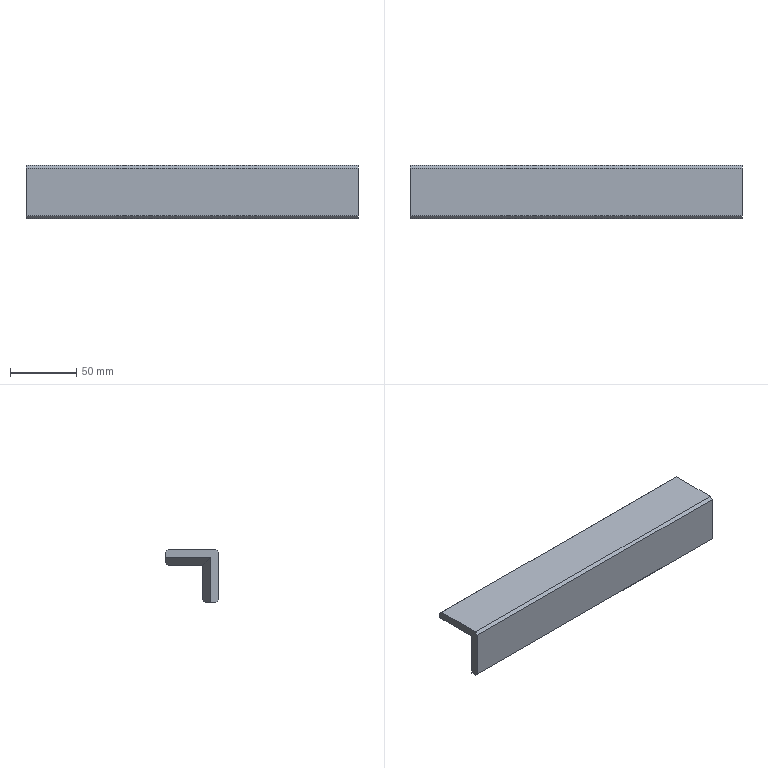Part | NX | 1 solid | 23 faces | box 250 x 40 x 40 mm | volume 198881 mm3 | plane 15 | cone 4 | cylinder 4 | commonest cylinder face diameters 4.2 x4
STEP:
#1=CARTESIAN_POINT('',(125.,-18.,20.));
#2=VERTEX_POINT('',#1);
#3=CARTESIAN_POINT('',(125.,-20.,18.));
#4=VERTEX_POINT('',#3);
#5=CARTESIAN_POINT('',(125.,-19.,19.));
#6=DIRECTION('',(0.,-0.7071,-0.7071));
#7=VECTOR('',#6,1000.);
#8=LINE('',#5,#7);
#9=EDGE_CURVE('',#2,#4,#8,.T.);
#10=ORIENTED_EDGE('',*,*,#9,.F.);
#11=CARTESIAN_POINT('',(-125.,-18.,20.));
#12=VERTEX_POINT('',#11);
#13=CARTESIAN_POINT('',(125.,-18.,20.));
#14=DIRECTION('',(1.,0.,0.));
#15=VECTOR('',#14,1000.);
#16=LINE('',#13,#15);
#17=EDGE_CURVE('',#12,#2,#16,.T.);
#18=ORIENTED_EDGE('',*,*,#17,.F.);
#19=CARTESIAN_POINT('',(-125.,-20.,18.));
#20=VERTEX_POINT('',#19);
#21=CARTESIAN_POINT('',(-125.,-20.,18.));
#22=DIRECTION('',(0.,0.7071,0.7071));
#23=VECTOR('',#22,1000.);
#24=LINE('',#21,#23);
#25=EDGE_CURVE('',#20,#12,#24,.T.);
#26=ORIENTED_EDGE('',*,*,#25,.F.);
#27=CARTESIAN_POINT('',(125.,-20.,18.));
#28=DIRECTION('',(-1.,0.,0.));
#29=VECTOR('',#28,1000.);
#30=LINE('',#27,#29);
#31=EDGE_CURVE('',#4,#20,#30,.T.);
#32=ORIENTED_EDGE('',*,*,#31,.F.);
#33=EDGE_LOOP('',(#10,#18,#26,#32));
#34=FACE_BOUND('',#33,.T.);
#35=CARTESIAN_POINT('',(125.,-20.,18.));
#36=DIRECTION('',(0.,0.7071,-0.7071));
#37=DIRECTION('',(-1.,0.,0.));
#38=AXIS2_PLACEMENT_3D('',#35,#36,#37);
#39=PLANE('',#38);
#40=ADVANCED_FACE('',(#34),#39,.F.);
#41=CARTESIAN_POINT('',(125.,-20.,-18.));
#42=VERTEX_POINT('',#41);
#43=CARTESIAN_POINT('',(125.,-18.,-20.));
#44=VERTEX_POINT('',#43);
#45=CARTESIAN_POINT('',(125.,-19.,-19.));
#46=DIRECTION('',(0.,0.7071,-0.7071));
#47=VECTOR('',#46,1000.);
#48=LINE('',#45,#47);
#49=EDGE_CURVE('',#42,#44,#48,.T.);
#50=ORIENTED_EDGE('',*,*,#49,.F.);
#51=CARTESIAN_POINT('',(-125.,-20.,-18.));
#52=VERTEX_POINT('',#51);
#53=CARTESIAN_POINT('',(125.,-20.,-18.));
#54=DIRECTION('',(1.,0.,0.));
#55=VECTOR('',#54,1000.);
#56=LINE('',#53,#55);
#57=EDGE_CURVE('',#52,#42,#56,.T.);
#58=ORIENTED_EDGE('',*,*,#57,.F.);
#59=CARTESIAN_POINT('',(-125.,-18.,-20.));
#60=VERTEX_POINT('',#59);
#61=CARTESIAN_POINT('',(-125.,-18.,-20.));
#62=DIRECTION('',(0.,-0.7071,0.7071));
#63=VECTOR('',#62,1000.);
#64=LINE('',#61,#63);
#65=EDGE_CURVE('',#60,#52,#64,.T.);
#66=ORIENTED_EDGE('',*,*,#65,.F.);
#67=CARTESIAN_POINT('',(125.,-18.,-20.));
#68=DIRECTION('',(-1.,0.,0.));
#69=VECTOR('',#68,1000.);
#70=LINE('',#67,#69);
#71=EDGE_CURVE('',#44,#60,#70,.T.);
#72=ORIENTED_EDGE('',*,*,#71,.F.);
#73=EDGE_LOOP('',(#50,#58,#66,#72));
#74=FACE_BOUND('',#73,.T.);
#75=CARTESIAN_POINT('',(125.,-18.,-20.));
#76=DIRECTION('',(0.,0.7071,0.7071));
#77=DIRECTION('',(-1.,0.,0.));
#78=AXIS2_PLACEMENT_3D('',#75,#76,#77);
#79=PLANE('',#78);
#80=ADVANCED_FACE('',(#74),#79,.F.);
#81=CARTESIAN_POINT('',(125.,20.,18.));
#82=VERTEX_POINT('',#81);
#83=CARTESIAN_POINT('',(125.,18.,20.));
#84=VERTEX_POINT('',#83);
#85=CARTESIAN_POINT('',(125.,19.,19.));
#86=DIRECTION('',(0.,-0.7071,0.7071));
#87=VECTOR('',#86,1000.);
#88=LINE('',#85,#87);
#89=EDGE_CURVE('',#82,#84,#88,.T.);
#90=ORIENTED_EDGE('',*,*,#89,.F.);
#91=CARTESIAN_POINT('',(-125.,20.,18.));
#92=VERTEX_POINT('',#91);
#93=CARTESIAN_POINT('',(125.,20.,18.));
#94=DIRECTION('',(1.,0.,0.));
#95=VECTOR('',#94,1000.);
#96=LINE('',#93,#95);
#97=EDGE_CURVE('',#92,#82,#96,.T.);
#98=ORIENTED_EDGE('',*,*,#97,.F.);
#99=CARTESIAN_POINT('',(-125.,18.,20.));
#100=VERTEX_POINT('',#99);
#101=CARTESIAN_POINT('',(-125.,18.,20.));
#102=DIRECTION('',(0.,0.7071,-0.7071));
#103=VECTOR('',#102,1000.);
#104=LINE('',#101,#103);
#105=EDGE_CURVE('',#100,#92,#104,.T.);
#106=ORIENTED_EDGE('',*,*,#105,.F.);
#107=CARTESIAN_POINT('',(125.,18.,20.));
#108=DIRECTION('',(-1.,0.,0.));
#109=VECTOR('',#108,1000.);
#110=LINE('',#107,#109);
#111=EDGE_CURVE('',#84,#100,#110,.T.);
#112=ORIENTED_EDGE('',*,*,#111,.F.);
#113=EDGE_LOOP('',(#90,#98,#106,#112));
#114=FACE_BOUND('',#113,.T.);
#115=CARTESIAN_POINT('',(125.,18.,20.));
#116=DIRECTION('',(0.,-0.7071,-0.7071));
#117=DIRECTION('',(-1.,0.,0.));
#118=AXIS2_PLACEMENT_3D('',#115,#116,#117);
#119=PLANE('',#118);
#120=ADVANCED_FACE('',(#114),#119,.F.);
#121=CARTESIAN_POINT('',(-118.333,20.,10.));
#122=VERTEX_POINT('',#121);
#123=CARTESIAN_POINT('',(-115.,18.,8.));
#124=VERTEX_POINT('',#123);
#125=CARTESIAN_POINT('',(-116.628,18.977,8.977));
#126=DIRECTION('',(0.7625,-0.4575,-0.4575));
#127=VECTOR('',#126,1000.);
#128=LINE('',#125,#127);
#129=EDGE_CURVE('',#122,#124,#128,.T.);
#130=ORIENTED_EDGE('',*,*,#129,.F.);
#131=CARTESIAN_POINT('',(125.,20.,10.));
#132=VERTEX_POINT('',#131);
#133=CARTESIAN_POINT('',(125.,20.,10.));
#134=DIRECTION('',(-1.,0.,0.));
#135=VECTOR('',#134,1000.);
#136=LINE('',#133,#135);
#137=EDGE_CURVE('',#132,#122,#136,.T.);
#138=ORIENTED_EDGE('',*,*,#137,.F.);
#139=CARTESIAN_POINT('',(125.,18.,8.));
#140=VERTEX_POINT('',#139);
#141=CARTESIAN_POINT('',(125.,5.,-5.));
#142=DIRECTION('',(0.,0.7071,0.7071));
#143=VECTOR('',#142,1000.);
#144=LINE('',#141,#143);
#145=EDGE_CURVE('',#140,#132,#144,.T.);
#146=ORIENTED_EDGE('',*,*,#145,.F.);
#147=CARTESIAN_POINT('',(-125.,18.,8.));
#148=DIRECTION('',(1.,0.,0.));
#149=VECTOR('',#148,1000.);
#150=LINE('',#147,#149);
#151=EDGE_CURVE('',#124,#140,#150,.T.);
#152=ORIENTED_EDGE('',*,*,#151,.F.);
#153=EDGE_LOOP('',(#130,#138,#146,#152));
#154=FACE_BOUND('',#153,.T.);
#155=CARTESIAN_POINT('',(125.,-10.,-20.));
#156=DIRECTION('',(0.,-0.7071,0.7071));
#157=DIRECTION('',(1.,0.,0.));
#158=AXIS2_PLACEMENT_3D('',#155,#156,#157);
#159=PLANE('',#158);
#160=ADVANCED_FACE('',(#154),#159,.F.);
#161=CARTESIAN_POINT('',(-115.,-8.,-18.));
#162=VERTEX_POINT('',#161);
#163=CARTESIAN_POINT('',(-118.333,-10.,-20.));
#164=VERTEX_POINT('',#163);
#165=CARTESIAN_POINT('',(-116.628,-8.977,-18.977));
#166=DIRECTION('',(-0.7625,-0.4575,-0.4575));
#167=VECTOR('',#166,1000.);
#168=LINE('',#165,#167);
#169=EDGE_CURVE('',#162,#164,#168,.T.);
#170=ORIENTED_EDGE('',*,*,#169,.F.);
#171=CARTESIAN_POINT('',(125.,-8.,-18.));
#172=VERTEX_POINT('',#171);
#173=CARTESIAN_POINT('',(-125.,-8.,-18.));
#174=DIRECTION('',(-1.,0.,0.));
#175=VECTOR('',#174,1000.);
#176=LINE('',#173,#175);
#177=EDGE_CURVE('',#172,#162,#176,.T.);
#178=ORIENTED_EDGE('',*,*,#177,.F.);
#179=CARTESIAN_POINT('',(125.,-10.,-20.));
#180=VERTEX_POINT('',#179);
#181=CARTESIAN_POINT('',(125.,5.,-5.));
#182=DIRECTION('',(0.,0.7071,0.7071));
#183=VECTOR('',#182,1000.);
#184=LINE('',#181,#183);
#185=EDGE_CURVE('',#180,#172,#184,.T.);
#186=ORIENTED_EDGE('',*,*,#185,.F.);
#187=CARTESIAN_POINT('',(125.,-10.,-20.));
#188=DIRECTION('',(1.,0.,0.));
#189=VECTOR('',#188,1000.);
#190=LINE('',#187,#189);
#191=EDGE_CURVE('',#164,#180,#190,.T.);
#192=ORIENTED_EDGE('',*,*,#191,.F.);
#193=EDGE_LOOP('',(#170,#178,#186,#192));
#194=FACE_BOUND('',#193,.T.);
#195=CARTESIAN_POINT('',(125.,-10.,-20.));
#196=DIRECTION('',(0.,-0.7071,0.7071));
#197=DIRECTION('',(1.,0.,0.));
#198=AXIS2_PLACEMENT_3D('',#195,#196,#197);
#199=PLANE('',#198);
#200=ADVANCED_FACE('',(#194),#199,.F.);
#201=CARTESIAN_POINT('',(-115.,-8.,8.));
#202=VERTEX_POINT('',#201);
#203=CARTESIAN_POINT('',(-115.,-8.,-20.));
#204=DIRECTION('',(0.,0.,1.));
#205=VECTOR('',#204,1000.);
#206=LINE('',#203,#205);
#207=EDGE_CURVE('',#162,#202,#206,.T.);
#208=ORIENTED_EDGE('',*,*,#207,.F.);
#209=ORIENTED_EDGE('',*,*,#169,.T.);
#210=CARTESIAN_POINT('',(-125.,-14.,-20.));
#211=VERTEX_POINT('',#210);
#212=CARTESIAN_POINT('',(-125.,-14.,-20.));
#213=DIRECTION('',(0.8575,0.5145,0.));
#214=VECTOR('',#213,1000.);
#215=LINE('',#212,#214);
#216=EDGE_CURVE('',#211,#164,#215,.T.);
#217=ORIENTED_EDGE('',*,*,#216,.F.);
#218=CARTESIAN_POINT('',(-125.,-14.,14.));
#219=VERTEX_POINT('',#218);
#220=CARTESIAN_POINT('',(-125.,-14.,0.));
#221=DIRECTION('',(0.,0.,-1.));
#222=VECTOR('',#221,1000.);
#223=LINE('',#220,#222);
#224=EDGE_CURVE('',#219,#211,#223,.T.);
#225=ORIENTED_EDGE('',*,*,#224,.F.);
#226=CARTESIAN_POINT('',(-120.116,-11.07,11.07));
#227=DIRECTION('',(0.7625,0.4575,-0.4575));
#228=VECTOR('',#227,1000.);
#229=LINE('',#226,#228);
#230=EDGE_CURVE('',#219,#202,#229,.T.);
#231=ORIENTED_EDGE('',*,*,#230,.T.);
#232=EDGE_LOOP('',(#208,#209,#217,#225,#231));
#233=FACE_BOUND('',#232,.T.);
#234=CARTESIAN_POINT('',(-125.,-14.,0.));
#235=DIRECTION('',(0.5145,-0.8575,0.));
#236=DIRECTION('',(0.,0.,-1.));
#237=AXIS2_PLACEMENT_3D('',#234,#235,#236);
#238=PLANE('',#237);
#239=ADVANCED_FACE('',(#233),#238,.F.);
#240=CARTESIAN_POINT('',(-125.,20.,14.));
#241=VERTEX_POINT('',#240);
#242=CARTESIAN_POINT('',(-125.,20.,14.));
#243=DIRECTION('',(-0.8575,0.,0.5145));
#244=VECTOR('',#243,1000.);
#245=LINE('',#242,#244);
#246=EDGE_CURVE('',#122,#241,#245,.T.);
#247=ORIENTED_EDGE('',*,*,#246,.F.);
#248=ORIENTED_EDGE('',*,*,#129,.T.);
#249=CARTESIAN_POINT('',(-115.,20.,8.));
#250=DIRECTION('',(0.,1.,0.));
#251=VECTOR('',#250,1000.);
#252=LINE('',#249,#251);
#253=EDGE_CURVE('',#202,#124,#252,.T.);
#254=ORIENTED_EDGE('',*,*,#253,.F.);
#255=ORIENTED_EDGE('',*,*,#230,.F.);
#256=CARTESIAN_POINT('',(-125.,0.,14.));
#257=DIRECTION('',(0.,-1.,0.));
#258=VECTOR('',#257,1000.);
#259=LINE('',#256,#258);
#260=EDGE_CURVE('',#241,#219,#259,.T.);
#261=ORIENTED_EDGE('',*,*,#260,.F.);
#262=EDGE_LOOP('',(#247,#248,#254,#255,#261));
#263=FACE_BOUND('',#262,.T.);
#264=CARTESIAN_POINT('',(-125.,0.,14.));
#265=DIRECTION('',(0.5145,0.,0.8575));
#266=DIRECTION('',(0.,-1.,0.));
#267=AXIS2_PLACEMENT_3D('',#264,#265,#266);
#268=PLANE('',#267);
#269=ADVANCED_FACE('',(#263),#268,.F.);
#270=ORIENTED_EDGE('',*,*,#253,.T.);
#271=ORIENTED_EDGE('',*,*,#151,.T.);
#272=CARTESIAN_POINT('',(125.,-8.,8.));
#273=VERTEX_POINT('',#272);
#274=CARTESIAN_POINT('',(125.,20.,8.));
#275=DIRECTION('',(0.,-1.,0.));
#276=VECTOR('',#275,1000.);
#277=LINE('',#274,#276);
#278=EDGE_CURVE('',#140,#273,#277,.T.);
#279=ORIENTED_EDGE('',*,*,#278,.T.);
#280=CARTESIAN_POINT('',(-125.,-8.,8.));
#281=DIRECTION('',(1.,0.,0.));
#282=VECTOR('',#281,1000.);
#283=LINE('',#280,#282);
#284=EDGE_CURVE('',#202,#273,#283,.T.);
#285=ORIENTED_EDGE('',*,*,#284,.F.);
#286=EDGE_LOOP('',(#270,#271,#279,#285));
#287=FACE_BOUND('',#286,.T.);
#288=CARTESIAN_POINT('',(-125.,20.,8.));
#289=DIRECTION('',(0.,0.,1.));
#290=DIRECTION('',(0.,-1.,0.));
#291=AXIS2_PLACEMENT_3D('',#288,#289,#290);
#292=PLANE('',#291);
#293=ADVANCED_FACE('',(#287),#292,.F.);
#294=CARTESIAN_POINT('',(125.,-8.,-20.));
#295=DIRECTION('',(0.,0.,-1.));
#296=VECTOR('',#295,1000.);
#297=LINE('',#294,#296);
#298=EDGE_CURVE('',#273,#172,#297,.T.);
#299=ORIENTED_EDGE('',*,*,#298,.T.);
#300=ORIENTED_EDGE('',*,*,#177,.T.);
#301=ORIENTED_EDGE('',*,*,#207,.T.);
#302=ORIENTED_EDGE('',*,*,#284,.T.);
#303=EDGE_LOOP('',(#299,#300,#301,#302));
#304=FACE_BOUND('',#303,.T.);
#305=CARTESIAN_POINT('',(-125.,-8.,-20.));
#306=DIRECTION('',(0.,-1.,0.));
#307=DIRECTION('',(0.,0.,-1.));
#308=AXIS2_PLACEMENT_3D('',#305,#306,#307);
#309=PLANE('',#308);
#310=ADVANCED_FACE('',(#304),#309,.F.);
#311=CARTESIAN_POINT('',(-125.,20.,20.));
#312=DIRECTION('',(0.,-1.,0.));
#313=VECTOR('',#312,1000.);
#314=LINE('',#311,#313);
#315=EDGE_CURVE('',#100,#12,#314,.T.);
#316=ORIENTED_EDGE('',*,*,#315,.F.);
#317=ORIENTED_EDGE('',*,*,#105,.T.);
#318=CARTESIAN_POINT('',(-125.,20.,20.));
#319=DIRECTION('',(0.,0.,1.));
#320=VECTOR('',#319,1000.);
#321=LINE('',#318,#320);
#322=EDGE_CURVE('',#241,#92,#321,.T.);
#323=ORIENTED_EDGE('',*,*,#322,.F.);
#324=ORIENTED_EDGE('',*,*,#260,.T.);
#325=ORIENTED_EDGE('',*,*,#224,.T.);
#326=CARTESIAN_POINT('',(-125.,20.,-20.));
#327=DIRECTION('',(0.,1.,0.));
#328=VECTOR('',#327,1000.);
#329=LINE('',#326,#328);
#330=EDGE_CURVE('',#60,#211,#329,.T.);
#331=ORIENTED_EDGE('',*,*,#330,.F.);
#332=ORIENTED_EDGE('',*,*,#65,.T.);
#333=CARTESIAN_POINT('',(-125.,-20.,20.));
#334=DIRECTION('',(0.,0.,-1.));
#335=VECTOR('',#334,1000.);
#336=LINE('',#333,#335);
#337=EDGE_CURVE('',#20,#52,#336,.T.);
#338=ORIENTED_EDGE('',*,*,#337,.F.);
#339=ORIENTED_EDGE('',*,*,#25,.T.);
#340=EDGE_LOOP('',(#316,#317,#323,#324,#325,#331,#332,#338,#339));
#341=FACE_BOUND('',#340,.T.);
#342=CARTESIAN_POINT('',(-125.,0.,0.));
#343=DIRECTION('',(1.,0.,0.));
#344=DIRECTION('',(0.,0.,-1.));
#345=AXIS2_PLACEMENT_3D('',#342,#343,#344);
#346=PLANE('',#345);
#347=ADVANCED_FACE('',(#341),#346,.F.);
#348=CARTESIAN_POINT('',(125.,20.,-20.));
#349=DIRECTION('',(0.,1.,0.));
#350=VECTOR('',#349,1000.);
#351=LINE('',#348,#350);
#352=EDGE_CURVE('',#44,#180,#351,.T.);
#353=ORIENTED_EDGE('',*,*,#352,.T.);
#354=ORIENTED_EDGE('',*,*,#185,.T.);
#355=ORIENTED_EDGE('',*,*,#298,.F.);
#356=ORIENTED_EDGE('',*,*,#278,.F.);
#357=ORIENTED_EDGE('',*,*,#145,.T.);
#358=CARTESIAN_POINT('',(125.,20.,20.));
#359=DIRECTION('',(0.,0.,1.));
#360=VECTOR('',#359,1000.);
#361=LINE('',#358,#360);
#362=EDGE_CURVE('',#132,#82,#361,.T.);
#363=ORIENTED_EDGE('',*,*,#362,.T.);
#364=ORIENTED_EDGE('',*,*,#89,.T.);
#365=CARTESIAN_POINT('',(125.,20.,20.));
#366=DIRECTION('',(0.,-1.,0.));
#367=VECTOR('',#366,1000.);
#368=LINE('',#365,#367);
#369=EDGE_CURVE('',#84,#2,#368,.T.);
#370=ORIENTED_EDGE('',*,*,#369,.T.);
#371=ORIENTED_EDGE('',*,*,#9,.T.);
#372=CARTESIAN_POINT('',(125.,-20.,20.));
#373=DIRECTION('',(0.,0.,-1.));
#374=VECTOR('',#373,1000.);
#375=LINE('',#372,#374);
#376=EDGE_CURVE('',#4,#42,#375,.T.);
#377=ORIENTED_EDGE('',*,*,#376,.T.);
#378=ORIENTED_EDGE('',*,*,#49,.T.);
#379=EDGE_LOOP('',(#353,#354,#355,#356,#357,#363,#364,#370,#371,#377,#378));
#380=FACE_BOUND('',#379,.T.);
#381=CARTESIAN_POINT('',(125.,14.,11.9));
#382=VERTEX_POINT('',#381);
#383=CARTESIAN_POINT('',(125.,14.,14.));
#384=DIRECTION('',(1.,0.,0.));
#385=DIRECTION('',(0.,0.,-1.));
#386=AXIS2_PLACEMENT_3D('',#383,#384,#385);
#387=CIRCLE('',#386,2.1);
#388=EDGE_CURVE('',#382,#382,#387,.T.);
#389=ORIENTED_EDGE('',*,*,#388,.F.);
#390=EDGE_LOOP('',(#389));
#391=FACE_BOUND('',#390,.T.);
#392=CARTESIAN_POINT('',(125.,-2.,11.9));
#393=VERTEX_POINT('',#392);
#394=CARTESIAN_POINT('',(125.,-2.,14.));
#395=DIRECTION('',(1.,0.,0.));
#396=DIRECTION('',(0.,0.,-1.));
#397=AXIS2_PLACEMENT_3D('',#394,#395,#396);
#398=CIRCLE('',#397,2.1);
#399=EDGE_CURVE('',#393,#393,#398,.T.);
#400=ORIENTED_EDGE('',*,*,#399,.F.);
#401=EDGE_LOOP('',(#400));
#402=FACE_BOUND('',#401,.T.);
#403=CARTESIAN_POINT('',(125.,-14.,-0.1));
#404=VERTEX_POINT('',#403);
#405=CARTESIAN_POINT('',(125.,-14.,2.));
#406=DIRECTION('',(1.,0.,0.));
#407=DIRECTION('',(0.,0.,-1.));
#408=AXIS2_PLACEMENT_3D('',#405,#406,#407);
#409=CIRCLE('',#408,2.1);
#410=EDGE_CURVE('',#404,#404,#409,.T.);
#411=ORIENTED_EDGE('',*,*,#410,.F.);
#412=EDGE_LOOP('',(#411));
#413=FACE_BOUND('',#412,.T.);
#414=CARTESIAN_POINT('',(125.,-14.,-16.1));
#415=VERTEX_POINT('',#414);
#416=CARTESIAN_POINT('',(125.,-14.,-14.));
#417=DIRECTION('',(1.,0.,0.));
#418=DIRECTION('',(0.,0.,-1.));
#419=AXIS2_PLACEMENT_3D('',#416,#417,#418);
#420=CIRCLE('',#419,2.1);
#421=EDGE_CURVE('',#415,#415,#420,.T.);
#422=ORIENTED_EDGE('',*,*,#421,.F.);
#423=EDGE_LOOP('',(#422));
#424=FACE_BOUND('',#423,.T.);
#425=CARTESIAN_POINT('',(125.,0.,0.));
#426=DIRECTION('',(1.,0.,0.));
#427=DIRECTION('',(0.,0.,-1.));
#428=AXIS2_PLACEMENT_3D('',#425,#426,#427);
#429=PLANE('',#428);
#430=ADVANCED_FACE('',(#380,#391,#402,#413,#424),#429,.T.);
#431=ORIENTED_EDGE('',*,*,#337,.T.);
#432=ORIENTED_EDGE('',*,*,#57,.T.);
#433=ORIENTED_EDGE('',*,*,#376,.F.);
#434=ORIENTED_EDGE('',*,*,#31,.T.);
#435=EDGE_LOOP('',(#431,#432,#433,#434));
#436=FACE_BOUND('',#435,.T.);
#437=CARTESIAN_POINT('',(125.,-20.,20.));
#438=DIRECTION('',(0.,1.,0.));
#439=DIRECTION('',(0.,0.,1.));
#440=AXIS2_PLACEMENT_3D('',#437,#438,#439);
#441=PLANE('',#440);
#442=ADVANCED_FACE('',(#436),#441,.F.);
#443=ORIENTED_EDGE('',*,*,#369,.F.);
#444=ORIENTED_EDGE('',*,*,#111,.T.);
#445=ORIENTED_EDGE('',*,*,#315,.T.);
#446=ORIENTED_EDGE('',*,*,#17,.T.);
#447=EDGE_LOOP('',(#443,#444,#445,#446));
#448=FACE_BOUND('',#447,.T.);
#449=CARTESIAN_POINT('',(125.,20.,20.));
#450=DIRECTION('',(0.,0.,-1.));
#451=DIRECTION('',(0.,1.,0.));
#452=AXIS2_PLACEMENT_3D('',#449,#450,#451);
#453=PLANE('',#452);
#454=ADVANCED_FACE('',(#448),#453,.F.);
#455=ORIENTED_EDGE('',*,*,#362,.F.);
#456=ORIENTED_EDGE('',*,*,#137,.T.);
#457=ORIENTED_EDGE('',*,*,#246,.T.);
#458=ORIENTED_EDGE('',*,*,#322,.T.);
#459=ORIENTED_EDGE('',*,*,#97,.T.);
#460=EDGE_LOOP('',(#455,#456,#457,#458,#459));
#461=FACE_BOUND('',#460,.T.);
#462=CARTESIAN_POINT('',(125.,20.,20.));
#463=DIRECTION('',(0.,-1.,0.));
#464=DIRECTION('',(0.,0.,-1.));
#465=AXIS2_PLACEMENT_3D('',#462,#463,#464);
#466=PLANE('',#465);
#467=ADVANCED_FACE('',(#461),#466,.F.);
#468=ORIENTED_EDGE('',*,*,#216,.T.);
#469=ORIENTED_EDGE('',*,*,#191,.T.);
#470=ORIENTED_EDGE('',*,*,#352,.F.);
#471=ORIENTED_EDGE('',*,*,#71,.T.);
#472=ORIENTED_EDGE('',*,*,#330,.T.);
#473=EDGE_LOOP('',(#468,#469,#470,#471,#472));
#474=FACE_BOUND('',#473,.T.);
#475=CARTESIAN_POINT('',(125.,20.,-20.));
#476=DIRECTION('',(0.,0.,1.));
#477=DIRECTION('',(0.,-1.,0.));
#478=AXIS2_PLACEMENT_3D('',#475,#476,#477);
#479=PLANE('',#478);
#480=ADVANCED_FACE('',(#474),#479,.F.);
#481=CARTESIAN_POINT('',(108.738,14.,14.));
#482=VERTEX_POINT('',#481);
#483=VERTEX_LOOP('',#482);
#484=FACE_BOUND('',#483,.T.);
#485=CARTESIAN_POINT('',(110.,14.,11.9));
#486=VERTEX_POINT('',#485);
#487=CARTESIAN_POINT('',(110.,14.,14.));
#488=DIRECTION('',(1.,0.,0.));
#489=DIRECTION('',(0.,0.,-1.));
#490=AXIS2_PLACEMENT_3D('',#487,#488,#489);
#491=CIRCLE('',#490,2.1);
#492=EDGE_CURVE('',#486,#486,#491,.T.);
#493=ORIENTED_EDGE('',*,*,#492,.T.);
#494=EDGE_LOOP('',(#493));
#495=FACE_BOUND('',#494,.T.);
#496=CARTESIAN_POINT('',(110.,14.,14.));
#497=DIRECTION('',(1.,0.,0.));
#498=DIRECTION('',(0.,0.,-1.));
#499=AXIS2_PLACEMENT_3D('',#496,#497,#498);
#500=CONICAL_SURFACE('',#499,2.1,1.03);
#501=ADVANCED_FACE('',(#484,#495),#500,.F.);
#502=ORIENTED_EDGE('',*,*,#388,.T.);
#503=EDGE_LOOP('',(#502));
#504=FACE_BOUND('',#503,.T.);
#505=ORIENTED_EDGE('',*,*,#492,.F.);
#506=EDGE_LOOP('',(#505));
#507=FACE_BOUND('',#506,.T.);
#508=CARTESIAN_POINT('',(125.,14.,14.));
#509=DIRECTION('',(1.,0.,0.));
#510=DIRECTION('',(0.,0.,-1.));
#511=AXIS2_PLACEMENT_3D('',#508,#509,#510);
#512=CYLINDRICAL_SURFACE('',#511,2.1);
#513=ADVANCED_FACE('',(#504,#507),#512,.F.);
#514=CARTESIAN_POINT('',(108.738,-2.,14.));
#515=VERTEX_POINT('',#514);
#516=VERTEX_LOOP('',#515);
#517=FACE_BOUND('',#516,.T.);
#518=CARTESIAN_POINT('',(110.,-2.,11.9));
#519=VERTEX_POINT('',#518);
#520=CARTESIAN_POINT('',(110.,-2.,14.));
#521=DIRECTION('',(1.,0.,0.));
#522=DIRECTION('',(0.,0.,-1.));
#523=AXIS2_PLACEMENT_3D('',#520,#521,#522);
#524=CIRCLE('',#523,2.1);
#525=EDGE_CURVE('',#519,#519,#524,.T.);
#526=ORIENTED_EDGE('',*,*,#525,.T.);
#527=EDGE_LOOP('',(#526));
#528=FACE_BOUND('',#527,.T.);
#529=CARTESIAN_POINT('',(110.,-2.,14.));
#530=DIRECTION('',(1.,0.,0.));
#531=DIRECTION('',(0.,0.,-1.));
#532=AXIS2_PLACEMENT_3D('',#529,#530,#531);
#533=CONICAL_SURFACE('',#532,2.1,1.03);
#534=ADVANCED_FACE('',(#517,#528),#533,.F.);
#535=ORIENTED_EDGE('',*,*,#399,.T.);
#536=EDGE_LOOP('',(#535));
#537=FACE_BOUND('',#536,.T.);
#538=ORIENTED_EDGE('',*,*,#525,.F.);
#539=EDGE_LOOP('',(#538));
#540=FACE_BOUND('',#539,.T.);
#541=CARTESIAN_POINT('',(125.,-2.,14.));
#542=DIRECTION('',(1.,0.,0.));
#543=DIRECTION('',(0.,0.,-1.));
#544=AXIS2_PLACEMENT_3D('',#541,#542,#543);
#545=CYLINDRICAL_SURFACE('',#544,2.1);
#546=ADVANCED_FACE('',(#537,#540),#545,.F.);
#547=CARTESIAN_POINT('',(108.738,-14.,2.));
#548=VERTEX_POINT('',#547);
#549=VERTEX_LOOP('',#548);
#550=FACE_BOUND('',#549,.T.);
#551=CARTESIAN_POINT('',(110.,-14.,-0.1));
#552=VERTEX_POINT('',#551);
#553=CARTESIAN_POINT('',(110.,-14.,2.));
#554=DIRECTION('',(1.,0.,0.));
#555=DIRECTION('',(0.,0.,-1.));
#556=AXIS2_PLACEMENT_3D('',#553,#554,#555);
#557=CIRCLE('',#556,2.1);
#558=EDGE_CURVE('',#552,#552,#557,.T.);
#559=ORIENTED_EDGE('',*,*,#558,.T.);
#560=EDGE_LOOP('',(#559));
#561=FACE_BOUND('',#560,.T.);
#562=CARTESIAN_POINT('',(110.,-14.,2.));
#563=DIRECTION('',(1.,0.,0.));
#564=DIRECTION('',(0.,0.,-1.));
#565=AXIS2_PLACEMENT_3D('',#562,#563,#564);
#566=CONICAL_SURFACE('',#565,2.1,1.03);
#567=ADVANCED_FACE('',(#550,#561),#566,.F.);
#568=ORIENTED_EDGE('',*,*,#410,.T.);
#569=EDGE_LOOP('',(#568));
#570=FACE_BOUND('',#569,.T.);
#571=ORIENTED_EDGE('',*,*,#558,.F.);
#572=EDGE_LOOP('',(#571));
#573=FACE_BOUND('',#572,.T.);
#574=CARTESIAN_POINT('',(125.,-14.,2.));
#575=DIRECTION('',(1.,0.,0.));
#576=DIRECTION('',(0.,0.,-1.));
#577=AXIS2_PLACEMENT_3D('',#574,#575,#576);
#578=CYLINDRICAL_SURFACE('',#577,2.1);
#579=ADVANCED_FACE('',(#570,#573),#578,.F.);
#580=CARTESIAN_POINT('',(108.738,-14.,-14.));
#581=VERTEX_POINT('',#580);
#582=VERTEX_LOOP('',#581);
#583=FACE_BOUND('',#582,.T.);
#584=CARTESIAN_POINT('',(110.,-14.,-16.1));
#585=VERTEX_POINT('',#584);
#586=CARTESIAN_POINT('',(110.,-14.,-14.));
#587=DIRECTION('',(1.,0.,0.));
#588=DIRECTION('',(0.,0.,-1.));
#589=AXIS2_PLACEMENT_3D('',#586,#587,#588);
#590=CIRCLE('',#589,2.1);
#591=EDGE_CURVE('',#585,#585,#590,.T.);
#592=ORIENTED_EDGE('',*,*,#591,.T.);
#593=EDGE_LOOP('',(#592));
#594=FACE_BOUND('',#593,.T.);
#595=CARTESIAN_POINT('',(110.,-14.,-14.));
#596=DIRECTION('',(1.,0.,0.));
#597=DIRECTION('',(0.,0.,-1.));
#598=AXIS2_PLACEMENT_3D('',#595,#596,#597);
#599=CONICAL_SURFACE('',#598,2.1,1.03);
#600=ADVANCED_FACE('',(#583,#594),#599,.F.);
#601=ORIENTED_EDGE('',*,*,#421,.T.);
#602=EDGE_LOOP('',(#601));
#603=FACE_BOUND('',#602,.T.);
#604=ORIENTED_EDGE('',*,*,#591,.F.);
#605=EDGE_LOOP('',(#604));
#606=FACE_BOUND('',#605,.T.);
#607=CARTESIAN_POINT('',(125.,-14.,-14.));
#608=DIRECTION('',(1.,0.,0.));
#609=DIRECTION('',(0.,0.,-1.));
#610=AXIS2_PLACEMENT_3D('',#607,#608,#609);
#611=CYLINDRICAL_SURFACE('',#610,2.1);
#612=ADVANCED_FACE('',(#603,#606),#611,.F.);
#613=CLOSED_SHELL('',(#40,#80,#120,#160,#200,#239,#269,#293,#310,#347,#430,#442,#454,#467,#480,#501,#513,#534,#546,#567,#579,#600,#612));
#614=MANIFOLD_SOLID_BREP('',#613);
#615=(LENGTH_UNIT()NAMED_UNIT(*)SI_UNIT(.MILLI.,.METRE.));
#616=UNCERTAINTY_MEASURE_WITH_UNIT(LENGTH_MEASURE(0.00001),#615,'','');
#617=(NAMED_UNIT(*)PLANE_ANGLE_UNIT()SI_UNIT($,.RADIAN.));
#618=(NAMED_UNIT(*)SI_UNIT($,.STERADIAN.)SOLID_ANGLE_UNIT());
#619=(GEOMETRIC_REPRESENTATION_CONTEXT(3)GLOBAL_UNCERTAINTY_ASSIGNED_CONTEXT((#616))GLOBAL_UNIT_ASSIGNED_CONTEXT((#615,#617,#618))REPRESENTATION_CONTEXT('',''));
#620=ADVANCED_BREP_SHAPE_REPRESENTATION('',(#614),#619);